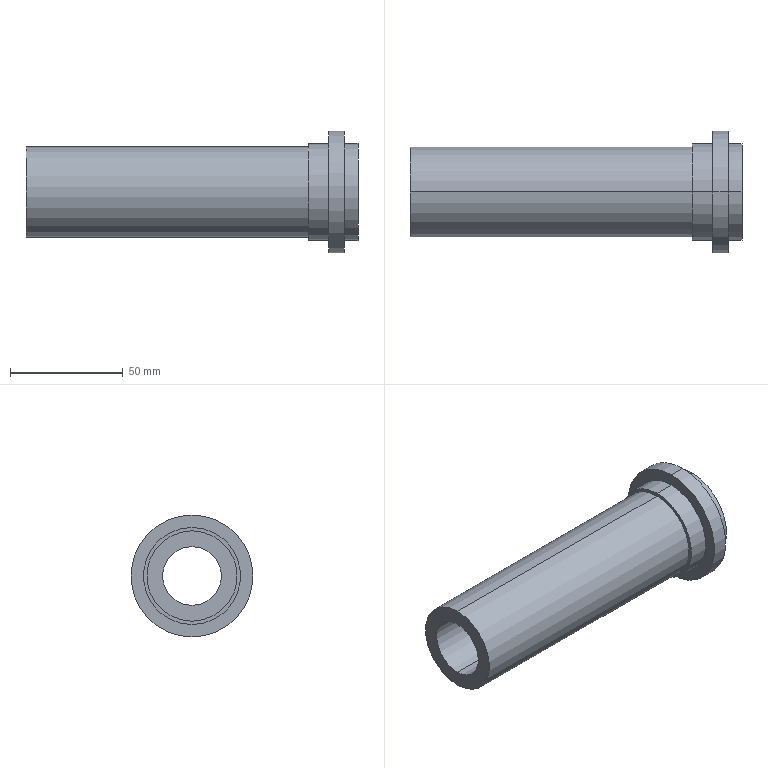Part | SolidWorks | features ICE 2, Revolution 1 | 1 solid | 15 faces | box 147 x 54 x 54 mm | volume 116848 mm3 | cylinder 10 | plane 5 | commonest cylinder face diameters 43 x4 26 x2 40 x2 54 x2
STEP:
#1=CARTESIAN_POINT('',(134.,0.,-27.));
#2=VERTEX_POINT('',#1);
#3=CARTESIAN_POINT('',(134.,0.,27.));
#4=VERTEX_POINT('',#3);
#5=CARTESIAN_POINT('',(134.,0.,0.));
#6=DIRECTION('',(1.,0.,0.));
#7=DIRECTION('',(0.,0.,-1.));
#8=AXIS2_PLACEMENT_3D('',#5,#6,#7);
#9=CIRCLE('',#8,27.);
#10=EDGE_CURVE('',#2,#4,#9,.T.);
#11=ORIENTED_EDGE('',*,*,#10,.T.);
#12=CARTESIAN_POINT('',(141.,0.,27.));
#13=VERTEX_POINT('',#12);
#14=CARTESIAN_POINT('',(134.,0.,27.));
#15=DIRECTION('',(1.,0.,0.));
#16=VECTOR('',#15,1000.);
#17=LINE('',#14,#16);
#18=EDGE_CURVE('',#4,#13,#17,.T.);
#19=ORIENTED_EDGE('',*,*,#18,.T.);
#20=CARTESIAN_POINT('',(141.,0.,-27.));
#21=VERTEX_POINT('',#20);
#22=CARTESIAN_POINT('',(141.,0.,0.));
#23=DIRECTION('',(1.,0.,0.));
#24=DIRECTION('',(0.,0.,-1.));
#25=AXIS2_PLACEMENT_3D('',#22,#23,#24);
#26=CIRCLE('',#25,27.);
#27=EDGE_CURVE('',#21,#13,#26,.T.);
#28=ORIENTED_EDGE('',*,*,#27,.F.);
#29=CARTESIAN_POINT('',(134.,0.,-27.));
#30=DIRECTION('',(1.,0.,0.));
#31=VECTOR('',#30,1000.);
#32=LINE('',#29,#31);
#33=EDGE_CURVE('',#2,#21,#32,.T.);
#34=ORIENTED_EDGE('',*,*,#33,.F.);
#35=EDGE_LOOP('',(#11,#19,#28,#34));
#36=FACE_OUTER_BOUND('',#35,.T.);
#37=CARTESIAN_POINT('',(134.,0.,0.));
#38=DIRECTION('',(1.,0.,0.));
#39=DIRECTION('',(0.,0.,-1.));
#40=AXIS2_PLACEMENT_3D('',#37,#38,#39);
#41=CYLINDRICAL_SURFACE('',#40,27.);
#42=ADVANCED_FACE('',(#36),#41,.T.);
#43=CARTESIAN_POINT('',(147.,0.,21.5));
#44=VERTEX_POINT('',#43);
#45=CARTESIAN_POINT('',(147.,0.,-21.5));
#46=VERTEX_POINT('',#45);
#47=CARTESIAN_POINT('',(147.,0.,0.));
#48=DIRECTION('',(-1.,0.,0.));
#49=DIRECTION('',(0.,0.,1.));
#50=AXIS2_PLACEMENT_3D('',#47,#48,#49);
#51=CIRCLE('',#50,21.5);
#52=EDGE_CURVE('',#44,#46,#51,.T.);
#53=ORIENTED_EDGE('',*,*,#52,.T.);
#54=CARTESIAN_POINT('',(141.,0.,-21.5));
#55=VERTEX_POINT('',#54);
#56=CARTESIAN_POINT('',(0.,0.,-21.5));
#57=DIRECTION('',(-1.,0.,0.));
#58=VECTOR('',#57,1000.);
#59=LINE('',#56,#58);
#60=EDGE_CURVE('',#46,#55,#59,.T.);
#61=ORIENTED_EDGE('',*,*,#60,.T.);
#62=CARTESIAN_POINT('',(141.,0.,21.5));
#63=VERTEX_POINT('',#62);
#64=CARTESIAN_POINT('',(141.,0.,0.));
#65=DIRECTION('',(1.,0.,0.));
#66=DIRECTION('',(0.,0.,-1.));
#67=AXIS2_PLACEMENT_3D('',#64,#65,#66);
#68=CIRCLE('',#67,21.5);
#69=EDGE_CURVE('',#55,#63,#68,.T.);
#70=ORIENTED_EDGE('',*,*,#69,.T.);
#71=CARTESIAN_POINT('',(0.,0.,21.5));
#72=DIRECTION('',(-1.,0.,0.));
#73=VECTOR('',#72,1000.);
#74=LINE('',#71,#73);
#75=EDGE_CURVE('',#44,#63,#74,.T.);
#76=ORIENTED_EDGE('',*,*,#75,.F.);
#77=EDGE_LOOP('',(#53,#61,#70,#76));
#78=FACE_OUTER_BOUND('',#77,.T.);
#79=CARTESIAN_POINT('',(0.,0.,0.));
#80=DIRECTION('',(-1.,0.,0.));
#81=DIRECTION('',(0.,0.,1.));
#82=AXIS2_PLACEMENT_3D('',#79,#80,#81);
#83=CYLINDRICAL_SURFACE('',#82,21.5);
#84=ADVANCED_FACE('',(#78),#83,.T.);
#85=CARTESIAN_POINT('',(125.,0.,20.));
#86=VERTEX_POINT('',#85);
#87=CARTESIAN_POINT('',(125.,0.,-20.));
#88=VERTEX_POINT('',#87);
#89=CARTESIAN_POINT('',(125.,0.,0.));
#90=DIRECTION('',(-1.,0.,0.));
#91=DIRECTION('',(0.,0.,1.));
#92=AXIS2_PLACEMENT_3D('',#89,#90,#91);
#93=CIRCLE('',#92,20.);
#94=EDGE_CURVE('',#86,#88,#93,.T.);
#95=ORIENTED_EDGE('',*,*,#94,.T.);
#96=CARTESIAN_POINT('',(0.,0.,-20.));
#97=VERTEX_POINT('',#96);
#98=CARTESIAN_POINT('',(0.,0.,-20.));
#99=DIRECTION('',(-1.,0.,0.));
#100=VECTOR('',#99,1000.);
#101=LINE('',#98,#100);
#102=EDGE_CURVE('',#88,#97,#101,.T.);
#103=ORIENTED_EDGE('',*,*,#102,.T.);
#104=CARTESIAN_POINT('',(0.,0.,20.));
#105=VERTEX_POINT('',#104);
#106=CARTESIAN_POINT('',(0.,0.,0.));
#107=DIRECTION('',(-1.,0.,0.));
#108=DIRECTION('',(0.,0.,1.));
#109=AXIS2_PLACEMENT_3D('',#106,#107,#108);
#110=CIRCLE('',#109,20.);
#111=EDGE_CURVE('',#105,#97,#110,.T.);
#112=ORIENTED_EDGE('',*,*,#111,.F.);
#113=CARTESIAN_POINT('',(0.,0.,20.));
#114=DIRECTION('',(-1.,0.,0.));
#115=VECTOR('',#114,1000.);
#116=LINE('',#113,#115);
#117=EDGE_CURVE('',#86,#105,#116,.T.);
#118=ORIENTED_EDGE('',*,*,#117,.F.);
#119=EDGE_LOOP('',(#95,#103,#112,#118));
#120=FACE_OUTER_BOUND('',#119,.T.);
#121=CARTESIAN_POINT('',(0.,0.,0.));
#122=DIRECTION('',(-1.,0.,0.));
#123=DIRECTION('',(0.,0.,1.));
#124=AXIS2_PLACEMENT_3D('',#121,#122,#123);
#125=CYLINDRICAL_SURFACE('',#124,20.);
#126=ADVANCED_FACE('',(#120),#125,.T.);
#127=CARTESIAN_POINT('',(147.,0.,-13.));
#128=VERTEX_POINT('',#127);
#129=CARTESIAN_POINT('',(147.,0.,13.));
#130=VERTEX_POINT('',#129);
#131=CARTESIAN_POINT('',(147.,0.,0.));
#132=DIRECTION('',(-1.,0.,0.));
#133=DIRECTION('',(0.,0.,1.));
#134=AXIS2_PLACEMENT_3D('',#131,#132,#133);
#135=CIRCLE('',#134,13.);
#136=EDGE_CURVE('',#128,#130,#135,.T.);
#137=ORIENTED_EDGE('',*,*,#136,.F.);
#138=CARTESIAN_POINT('',(0.,0.,-13.));
#139=VERTEX_POINT('',#138);
#140=CARTESIAN_POINT('',(0.,0.,-13.));
#141=DIRECTION('',(-1.,0.,0.));
#142=VECTOR('',#141,1000.);
#143=LINE('',#140,#142);
#144=EDGE_CURVE('',#128,#139,#143,.T.);
#145=ORIENTED_EDGE('',*,*,#144,.T.);
#146=CARTESIAN_POINT('',(0.,0.,13.));
#147=VERTEX_POINT('',#146);
#148=CARTESIAN_POINT('',(0.,0.,0.));
#149=DIRECTION('',(-1.,0.,0.));
#150=DIRECTION('',(0.,0.,1.));
#151=AXIS2_PLACEMENT_3D('',#148,#149,#150);
#152=CIRCLE('',#151,13.);
#153=EDGE_CURVE('',#139,#147,#152,.T.);
#154=ORIENTED_EDGE('',*,*,#153,.T.);
#155=CARTESIAN_POINT('',(0.,0.,13.));
#156=DIRECTION('',(-1.,0.,0.));
#157=VECTOR('',#156,1000.);
#158=LINE('',#155,#157);
#159=EDGE_CURVE('',#130,#147,#158,.T.);
#160=ORIENTED_EDGE('',*,*,#159,.F.);
#161=EDGE_LOOP('',(#137,#145,#154,#160));
#162=FACE_OUTER_BOUND('',#161,.T.);
#163=CARTESIAN_POINT('',(0.,0.,0.));
#164=DIRECTION('',(-1.,0.,0.));
#165=DIRECTION('',(0.,0.,1.));
#166=AXIS2_PLACEMENT_3D('',#163,#164,#165);
#167=CYLINDRICAL_SURFACE('',#166,13.);
#168=ADVANCED_FACE('',(#162),#167,.F.);
#169=CARTESIAN_POINT('',(134.,0.,-21.5));
#170=VERTEX_POINT('',#169);
#171=CARTESIAN_POINT('',(134.,0.,21.5));
#172=VERTEX_POINT('',#171);
#173=CARTESIAN_POINT('',(134.,0.,0.));
#174=DIRECTION('',(1.,0.,0.));
#175=DIRECTION('',(0.,0.,-1.));
#176=AXIS2_PLACEMENT_3D('',#173,#174,#175);
#177=CIRCLE('',#176,21.5);
#178=EDGE_CURVE('',#170,#172,#177,.T.);
#179=ORIENTED_EDGE('',*,*,#178,.F.);
#180=CARTESIAN_POINT('',(125.,0.,-21.5));
#181=VERTEX_POINT('',#180);
#182=CARTESIAN_POINT('',(0.,0.,-21.5));
#183=DIRECTION('',(-1.,0.,0.));
#184=VECTOR('',#183,1000.);
#185=LINE('',#182,#184);
#186=EDGE_CURVE('',#170,#181,#185,.T.);
#187=ORIENTED_EDGE('',*,*,#186,.T.);
#188=CARTESIAN_POINT('',(125.,0.,21.5));
#189=VERTEX_POINT('',#188);
#190=CARTESIAN_POINT('',(125.,0.,0.));
#191=DIRECTION('',(-1.,0.,0.));
#192=DIRECTION('',(0.,0.,1.));
#193=AXIS2_PLACEMENT_3D('',#190,#191,#192);
#194=CIRCLE('',#193,21.5);
#195=EDGE_CURVE('',#189,#181,#194,.T.);
#196=ORIENTED_EDGE('',*,*,#195,.F.);
#197=CARTESIAN_POINT('',(0.,0.,21.5));
#198=DIRECTION('',(-1.,0.,0.));
#199=VECTOR('',#198,1000.);
#200=LINE('',#197,#199);
#201=EDGE_CURVE('',#172,#189,#200,.T.);
#202=ORIENTED_EDGE('',*,*,#201,.F.);
#203=EDGE_LOOP('',(#179,#187,#196,#202));
#204=FACE_OUTER_BOUND('',#203,.T.);
#205=CARTESIAN_POINT('',(0.,0.,0.));
#206=DIRECTION('',(-1.,0.,0.));
#207=DIRECTION('',(0.,0.,1.));
#208=AXIS2_PLACEMENT_3D('',#205,#206,#207);
#209=CYLINDRICAL_SURFACE('',#208,21.5);
#210=ADVANCED_FACE('',(#204),#209,.T.);
#211=ORIENTED_EDGE('',*,*,#186,.F.);
#212=CARTESIAN_POINT('',(134.,0.,0.));
#213=DIRECTION('',(1.,0.,0.));
#214=DIRECTION('',(0.,0.,-1.));
#215=AXIS2_PLACEMENT_3D('',#212,#213,#214);
#216=CIRCLE('',#215,21.5);
#217=EDGE_CURVE('',#172,#170,#216,.T.);
#218=ORIENTED_EDGE('',*,*,#217,.F.);
#219=ORIENTED_EDGE('',*,*,#201,.T.);
#220=CARTESIAN_POINT('',(125.,0.,0.));
#221=DIRECTION('',(-1.,0.,0.));
#222=DIRECTION('',(0.,0.,1.));
#223=AXIS2_PLACEMENT_3D('',#220,#221,#222);
#224=CIRCLE('',#223,21.5);
#225=EDGE_CURVE('',#181,#189,#224,.T.);
#226=ORIENTED_EDGE('',*,*,#225,.F.);
#227=EDGE_LOOP('',(#211,#218,#219,#226));
#228=FACE_OUTER_BOUND('',#227,.T.);
#229=CARTESIAN_POINT('',(0.,0.,0.));
#230=DIRECTION('',(-1.,0.,0.));
#231=DIRECTION('',(0.,0.,1.));
#232=AXIS2_PLACEMENT_3D('',#229,#230,#231);
#233=CYLINDRICAL_SURFACE('',#232,21.5);
#234=ADVANCED_FACE('',(#228),#233,.T.);
#235=ORIENTED_EDGE('',*,*,#144,.F.);
#236=CARTESIAN_POINT('',(147.,0.,0.));
#237=DIRECTION('',(-1.,0.,0.));
#238=DIRECTION('',(0.,0.,1.));
#239=AXIS2_PLACEMENT_3D('',#236,#237,#238);
#240=CIRCLE('',#239,13.);
#241=EDGE_CURVE('',#130,#128,#240,.T.);
#242=ORIENTED_EDGE('',*,*,#241,.F.);
#243=ORIENTED_EDGE('',*,*,#159,.T.);
#244=CARTESIAN_POINT('',(0.,0.,0.));
#245=DIRECTION('',(-1.,0.,0.));
#246=DIRECTION('',(0.,0.,1.));
#247=AXIS2_PLACEMENT_3D('',#244,#245,#246);
#248=CIRCLE('',#247,13.);
#249=EDGE_CURVE('',#147,#139,#248,.T.);
#250=ORIENTED_EDGE('',*,*,#249,.T.);
#251=EDGE_LOOP('',(#235,#242,#243,#250));
#252=FACE_OUTER_BOUND('',#251,.T.);
#253=CARTESIAN_POINT('',(0.,0.,0.));
#254=DIRECTION('',(-1.,0.,0.));
#255=DIRECTION('',(0.,0.,1.));
#256=AXIS2_PLACEMENT_3D('',#253,#254,#255);
#257=CYLINDRICAL_SURFACE('',#256,13.);
#258=ADVANCED_FACE('',(#252),#257,.F.);
#259=ORIENTED_EDGE('',*,*,#249,.F.);
#260=ORIENTED_EDGE('',*,*,#153,.F.);
#261=EDGE_LOOP('',(#259,#260));
#262=FACE_BOUND('',#261,.T.);
#263=ORIENTED_EDGE('',*,*,#111,.T.);
#264=CARTESIAN_POINT('',(0.,0.,0.));
#265=DIRECTION('',(-1.,0.,0.));
#266=DIRECTION('',(0.,0.,1.));
#267=AXIS2_PLACEMENT_3D('',#264,#265,#266);
#268=CIRCLE('',#267,20.);
#269=EDGE_CURVE('',#97,#105,#268,.T.);
#270=ORIENTED_EDGE('',*,*,#269,.T.);
#271=EDGE_LOOP('',(#263,#270));
#272=FACE_OUTER_BOUND('',#271,.T.);
#273=CARTESIAN_POINT('',(0.,13.,0.));
#274=DIRECTION('',(1.,0.,0.));
#275=DIRECTION('',(0.,0.,-1.));
#276=AXIS2_PLACEMENT_3D('',#273,#274,#275);
#277=PLANE('',#276);
#278=ADVANCED_FACE('',(#262,#272),#277,.F.);
#279=ORIENTED_EDGE('',*,*,#102,.F.);
#280=CARTESIAN_POINT('',(125.,0.,0.));
#281=DIRECTION('',(-1.,0.,0.));
#282=DIRECTION('',(0.,0.,1.));
#283=AXIS2_PLACEMENT_3D('',#280,#281,#282);
#284=CIRCLE('',#283,20.);
#285=EDGE_CURVE('',#88,#86,#284,.T.);
#286=ORIENTED_EDGE('',*,*,#285,.T.);
#287=ORIENTED_EDGE('',*,*,#117,.T.);
#288=ORIENTED_EDGE('',*,*,#269,.F.);
#289=EDGE_LOOP('',(#279,#286,#287,#288));
#290=FACE_OUTER_BOUND('',#289,.T.);
#291=CARTESIAN_POINT('',(0.,0.,0.));
#292=DIRECTION('',(-1.,0.,0.));
#293=DIRECTION('',(0.,0.,1.));
#294=AXIS2_PLACEMENT_3D('',#291,#292,#293);
#295=CYLINDRICAL_SURFACE('',#294,20.);
#296=ADVANCED_FACE('',(#290),#295,.T.);
#297=ORIENTED_EDGE('',*,*,#94,.F.);
#298=ORIENTED_EDGE('',*,*,#285,.F.);
#299=EDGE_LOOP('',(#297,#298));
#300=FACE_BOUND('',#299,.T.);
#301=ORIENTED_EDGE('',*,*,#195,.T.);
#302=ORIENTED_EDGE('',*,*,#225,.T.);
#303=EDGE_LOOP('',(#301,#302));
#304=FACE_OUTER_BOUND('',#303,.T.);
#305=CARTESIAN_POINT('',(125.,20.,0.));
#306=DIRECTION('',(1.,0.,0.));
#307=DIRECTION('',(0.,0.,-1.));
#308=AXIS2_PLACEMENT_3D('',#305,#306,#307);
#309=PLANE('',#308);
#310=ADVANCED_FACE('',(#300,#304),#309,.F.);
#311=ORIENTED_EDGE('',*,*,#60,.F.);
#312=CARTESIAN_POINT('',(147.,0.,0.));
#313=DIRECTION('',(-1.,0.,0.));
#314=DIRECTION('',(0.,0.,1.));
#315=AXIS2_PLACEMENT_3D('',#312,#313,#314);
#316=CIRCLE('',#315,21.5);
#317=EDGE_CURVE('',#46,#44,#316,.T.);
#318=ORIENTED_EDGE('',*,*,#317,.T.);
#319=ORIENTED_EDGE('',*,*,#75,.T.);
#320=CARTESIAN_POINT('',(141.,0.,0.));
#321=DIRECTION('',(1.,0.,0.));
#322=DIRECTION('',(0.,0.,-1.));
#323=AXIS2_PLACEMENT_3D('',#320,#321,#322);
#324=CIRCLE('',#323,21.5);
#325=EDGE_CURVE('',#63,#55,#324,.T.);
#326=ORIENTED_EDGE('',*,*,#325,.T.);
#327=EDGE_LOOP('',(#311,#318,#319,#326));
#328=FACE_OUTER_BOUND('',#327,.T.);
#329=CARTESIAN_POINT('',(0.,0.,0.));
#330=DIRECTION('',(-1.,0.,0.));
#331=DIRECTION('',(0.,0.,1.));
#332=AXIS2_PLACEMENT_3D('',#329,#330,#331);
#333=CYLINDRICAL_SURFACE('',#332,21.5);
#334=ADVANCED_FACE('',(#328),#333,.T.);
#335=ORIENTED_EDGE('',*,*,#52,.F.);
#336=ORIENTED_EDGE('',*,*,#317,.F.);
#337=EDGE_LOOP('',(#335,#336));
#338=FACE_OUTER_BOUND('',#337,.T.);
#339=ORIENTED_EDGE('',*,*,#241,.T.);
#340=ORIENTED_EDGE('',*,*,#136,.T.);
#341=EDGE_LOOP('',(#339,#340));
#342=FACE_BOUND('',#341,.T.);
#343=CARTESIAN_POINT('',(147.,21.5,0.));
#344=DIRECTION('',(-1.,0.,0.));
#345=DIRECTION('',(0.,0.,1.));
#346=AXIS2_PLACEMENT_3D('',#343,#344,#345);
#347=PLANE('',#346);
#348=ADVANCED_FACE('',(#338,#342),#347,.F.);
#349=ORIENTED_EDGE('',*,*,#18,.F.);
#350=CARTESIAN_POINT('',(134.,0.,0.));
#351=DIRECTION('',(1.,0.,0.));
#352=DIRECTION('',(0.,0.,-1.));
#353=AXIS2_PLACEMENT_3D('',#350,#351,#352);
#354=CIRCLE('',#353,27.);
#355=EDGE_CURVE('',#4,#2,#354,.T.);
#356=ORIENTED_EDGE('',*,*,#355,.T.);
#357=ORIENTED_EDGE('',*,*,#33,.T.);
#358=CARTESIAN_POINT('',(141.,0.,0.));
#359=DIRECTION('',(1.,0.,0.));
#360=DIRECTION('',(0.,0.,-1.));
#361=AXIS2_PLACEMENT_3D('',#358,#359,#360);
#362=CIRCLE('',#361,27.);
#363=EDGE_CURVE('',#13,#21,#362,.T.);
#364=ORIENTED_EDGE('',*,*,#363,.F.);
#365=EDGE_LOOP('',(#349,#356,#357,#364));
#366=FACE_OUTER_BOUND('',#365,.T.);
#367=CARTESIAN_POINT('',(134.,0.,0.));
#368=DIRECTION('',(1.,0.,0.));
#369=DIRECTION('',(0.,0.,-1.));
#370=AXIS2_PLACEMENT_3D('',#367,#368,#369);
#371=CYLINDRICAL_SURFACE('',#370,27.);
#372=ADVANCED_FACE('',(#366),#371,.T.);
#373=ORIENTED_EDGE('',*,*,#217,.T.);
#374=ORIENTED_EDGE('',*,*,#178,.T.);
#375=EDGE_LOOP('',(#373,#374));
#376=FACE_BOUND('',#375,.T.);
#377=ORIENTED_EDGE('',*,*,#10,.F.);
#378=ORIENTED_EDGE('',*,*,#355,.F.);
#379=EDGE_LOOP('',(#377,#378));
#380=FACE_OUTER_BOUND('',#379,.T.);
#381=CARTESIAN_POINT('',(134.,0.,0.));
#382=DIRECTION('',(1.,0.,0.));
#383=DIRECTION('',(0.,0.,-1.));
#384=AXIS2_PLACEMENT_3D('',#381,#382,#383);
#385=PLANE('',#384);
#386=ADVANCED_FACE('',(#376,#380),#385,.F.);
#387=ORIENTED_EDGE('',*,*,#325,.F.);
#388=ORIENTED_EDGE('',*,*,#69,.F.);
#389=EDGE_LOOP('',(#387,#388));
#390=FACE_BOUND('',#389,.T.);
#391=ORIENTED_EDGE('',*,*,#27,.T.);
#392=ORIENTED_EDGE('',*,*,#363,.T.);
#393=EDGE_LOOP('',(#391,#392));
#394=FACE_OUTER_BOUND('',#393,.T.);
#395=CARTESIAN_POINT('',(141.,0.,0.));
#396=DIRECTION('',(1.,0.,0.));
#397=DIRECTION('',(0.,0.,-1.));
#398=AXIS2_PLACEMENT_3D('',#395,#396,#397);
#399=PLANE('',#398);
#400=ADVANCED_FACE('',(#390,#394),#399,.T.);
#401=CLOSED_SHELL('',(#42,#84,#126,#168,#210,#234,#258,#278,#296,#310,#334,#348,#372,#386,#400));
#402=MANIFOLD_SOLID_BREP('',#401);
#403=CARTESIAN_POINT('',(0.,0.,0.));
#404=DIRECTION('',(0.,0.,1.));
#405=DIRECTION('',(1.,0.,0.));
#406=AXIS2_PLACEMENT_3D('',#403,#404,#405);
#407=(LENGTH_UNIT()NAMED_UNIT(*)SI_UNIT(.MILLI.,.METRE.));
#408=UNCERTAINTY_MEASURE_WITH_UNIT(LENGTH_MEASURE(0.00001),#407,'','');
#409=(NAMED_UNIT(*)PLANE_ANGLE_UNIT()SI_UNIT($,.RADIAN.));
#410=(NAMED_UNIT(*)SI_UNIT($,.STERADIAN.)SOLID_ANGLE_UNIT());
#411=(GEOMETRIC_REPRESENTATION_CONTEXT(3)GLOBAL_UNCERTAINTY_ASSIGNED_CONTEXT((#408))GLOBAL_UNIT_ASSIGNED_CONTEXT((#407,#409,#410))REPRESENTATION_CONTEXT('',''));
#412=ADVANCED_BREP_SHAPE_REPRESENTATION('',(#402,#406),#411);